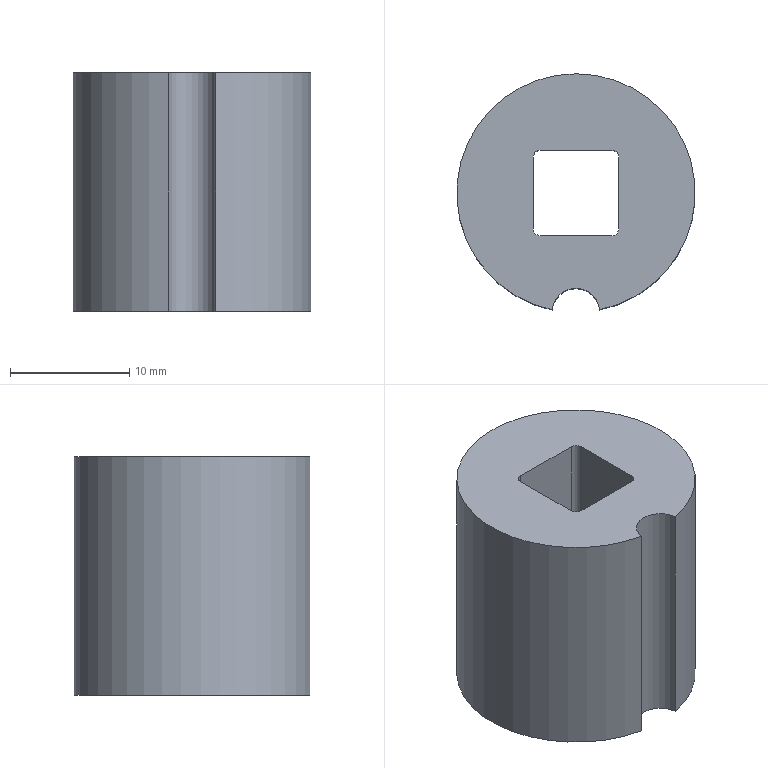Part | NX | features solid 2 | 1 solid | 14 faces | box 20 x 19.802 x 20 mm | volume 4258 mm3 | plane 7 | cylinder 7 | commonest cylinder face diameters 1.17 x4 4 x1 12.6 x1 20 x1
STEP:
#1=CARTESIAN_POINT('',(681.984,-23.915,28.23));
#2=VERTEX_POINT('',#1);
#3=CARTESIAN_POINT('',(678.004,-23.911,28.23));
#4=VERTEX_POINT('',#3);
#5=CARTESIAN_POINT('',(679.993,-24.113,28.23));
#6=DIRECTION('',(0.,0.,1.));
#7=DIRECTION('',(0.001096,1.,0.));
#8=AXIS2_PLACEMENT_3D('',#5,#6,#7);
#9=CIRCLE('',#8,2.);
#10=EDGE_CURVE('',#2,#4,#9,.T.);
#11=ORIENTED_EDGE('',*,*,#10,.F.);
#12=CARTESIAN_POINT('',(680.004,-14.113,28.23));
#13=DIRECTION('',(0.,0.,1.));
#14=DIRECTION('',(0.001096,1.,0.));
#15=AXIS2_PLACEMENT_3D('',#12,#13,#14);
#16=CIRCLE('',#15,10.);
#17=EDGE_CURVE('',#2,#4,#16,.T.);
#18=ORIENTED_EDGE('',*,*,#17,.T.);
#19=EDGE_LOOP('',(#11,#18));
#20=FACE_BOUND('',#19,.T.);
#21=CARTESIAN_POINT('',(677.001,-17.695,28.23));
#22=VERTEX_POINT('',#21);
#23=CARTESIAN_POINT('',(676.416,-17.109,28.23));
#24=VERTEX_POINT('',#23);
#25=CARTESIAN_POINT('',(677.001,-17.11,28.23));
#26=DIRECTION('',(0.,0.,-1.));
#27=DIRECTION('',(-1.,0.,0.));
#28=AXIS2_PLACEMENT_3D('',#25,#26,#27);
#29=CIRCLE('',#28,0.585);
#30=EDGE_CURVE('',#22,#24,#29,.T.);
#31=ORIENTED_EDGE('',*,*,#30,.T.);
#32=CARTESIAN_POINT('',(676.423,-11.109,28.23));
#33=VERTEX_POINT('',#32);
#34=CARTESIAN_POINT('',(676.419,-14.109,28.23));
#35=DIRECTION('',(-0.001096,-1.,0.));
#36=VECTOR('',#35,1000.);
#37=LINE('',#34,#36);
#38=EDGE_CURVE('',#33,#24,#37,.T.);
#39=ORIENTED_EDGE('',*,*,#38,.F.);
#40=CARTESIAN_POINT('',(677.008,-10.525,28.23));
#41=VERTEX_POINT('',#40);
#42=CARTESIAN_POINT('',(677.008,-11.11,28.23));
#43=DIRECTION('',(0.,0.,-1.));
#44=DIRECTION('',(-1.,0.,0.));
#45=AXIS2_PLACEMENT_3D('',#42,#43,#44);
#46=CIRCLE('',#45,0.585);
#47=EDGE_CURVE('',#33,#41,#46,.T.);
#48=ORIENTED_EDGE('',*,*,#47,.T.);
#49=CARTESIAN_POINT('',(683.008,-10.531,28.23));
#50=VERTEX_POINT('',#49);
#51=CARTESIAN_POINT('',(680.008,-10.528,28.23));
#52=DIRECTION('',(-1.,0.001096,0.));
#53=VECTOR('',#52,1000.);
#54=LINE('',#51,#53);
#55=EDGE_CURVE('',#50,#41,#54,.T.);
#56=ORIENTED_EDGE('',*,*,#55,.F.);
#57=CARTESIAN_POINT('',(683.593,-11.117,28.23));
#58=VERTEX_POINT('',#57);
#59=CARTESIAN_POINT('',(683.008,-11.116,28.23));
#60=DIRECTION('',(0.,0.,-1.));
#61=DIRECTION('',(-1.,0.,0.));
#62=AXIS2_PLACEMENT_3D('',#59,#60,#61);
#63=CIRCLE('',#62,0.585);
#64=EDGE_CURVE('',#50,#58,#63,.T.);
#65=ORIENTED_EDGE('',*,*,#64,.T.);
#66=CARTESIAN_POINT('',(683.586,-17.117,28.23));
#67=VERTEX_POINT('',#66);
#68=CARTESIAN_POINT('',(683.589,-14.117,28.23));
#69=DIRECTION('',(0.001096,1.,0.));
#70=VECTOR('',#69,1000.);
#71=LINE('',#68,#70);
#72=EDGE_CURVE('',#67,#58,#71,.T.);
#73=ORIENTED_EDGE('',*,*,#72,.F.);
#74=CARTESIAN_POINT('',(683.001,-17.701,28.23));
#75=VERTEX_POINT('',#74);
#76=CARTESIAN_POINT('',(683.001,-17.116,28.23));
#77=DIRECTION('',(0.,0.,-1.));
#78=DIRECTION('',(-1.,0.,0.));
#79=AXIS2_PLACEMENT_3D('',#76,#77,#78);
#80=CIRCLE('',#79,0.585);
#81=EDGE_CURVE('',#67,#75,#80,.T.);
#82=ORIENTED_EDGE('',*,*,#81,.T.);
#83=CARTESIAN_POINT('',(680.001,-17.698,28.23));
#84=DIRECTION('',(1.,-0.001096,0.));
#85=VECTOR('',#84,1000.);
#86=LINE('',#83,#85);
#87=EDGE_CURVE('',#22,#75,#86,.T.);
#88=ORIENTED_EDGE('',*,*,#87,.F.);
#89=EDGE_LOOP('',(#31,#39,#48,#56,#65,#73,#82,#88));
#90=FACE_BOUND('',#89,.T.);
#91=CARTESIAN_POINT('',(680.004,-14.113,28.23));
#92=DIRECTION('',(0.,0.,1.));
#93=DIRECTION('',(-0.001096,-1.,0.));
#94=AXIS2_PLACEMENT_3D('',#91,#92,#93);
#95=PLANE('',#94);
#96=ADVANCED_FACE('',(#20,#90),#95,.T.);
#97=CARTESIAN_POINT('',(678.004,-23.911,8.23));
#98=VERTEX_POINT('',#97);
#99=CARTESIAN_POINT('',(681.984,-23.915,8.23));
#100=VERTEX_POINT('',#99);
#101=CARTESIAN_POINT('',(679.993,-24.113,8.23));
#102=DIRECTION('',(0.,0.,-1.));
#103=DIRECTION('',(-0.001096,-1.,0.));
#104=AXIS2_PLACEMENT_3D('',#101,#102,#103);
#105=CIRCLE('',#104,2.);
#106=EDGE_CURVE('',#98,#100,#105,.T.);
#107=ORIENTED_EDGE('',*,*,#106,.F.);
#108=CARTESIAN_POINT('',(680.004,-14.113,8.23));
#109=DIRECTION('',(0.,0.,-1.));
#110=DIRECTION('',(-0.001096,-1.,0.));
#111=AXIS2_PLACEMENT_3D('',#108,#109,#110);
#112=CIRCLE('',#111,10.);
#113=EDGE_CURVE('',#98,#100,#112,.T.);
#114=ORIENTED_EDGE('',*,*,#113,.T.);
#115=EDGE_LOOP('',(#107,#114));
#116=FACE_BOUND('',#115,.T.);
#117=CARTESIAN_POINT('',(679.998,-20.413,8.23));
#118=VERTEX_POINT('',#117);
#119=CARTESIAN_POINT('',(680.004,-14.113,8.23));
#120=DIRECTION('',(0.,0.,-1.));
#121=DIRECTION('',(-0.001096,-1.,0.));
#122=AXIS2_PLACEMENT_3D('',#119,#120,#121);
#123=CIRCLE('',#122,6.3);
#124=EDGE_CURVE('',#118,#118,#123,.T.);
#125=ORIENTED_EDGE('',*,*,#124,.F.);
#126=EDGE_LOOP('',(#125));
#127=FACE_BOUND('',#126,.T.);
#128=CARTESIAN_POINT('',(680.004,-14.113,8.23));
#129=DIRECTION('',(0.,0.,-1.));
#130=DIRECTION('',(0.001096,1.,0.));
#131=AXIS2_PLACEMENT_3D('',#128,#129,#130);
#132=PLANE('',#131);
#133=ADVANCED_FACE('',(#116,#127),#132,.T.);
#134=CARTESIAN_POINT('',(678.004,-23.911,18.23));
#135=DIRECTION('',(0.,0.,1.));
#136=VECTOR('',#135,1000.);
#137=LINE('',#134,#136);
#138=EDGE_CURVE('',#98,#4,#137,.T.);
#139=ORIENTED_EDGE('',*,*,#138,.T.);
#140=ORIENTED_EDGE('',*,*,#17,.F.);
#141=CARTESIAN_POINT('',(681.984,-23.915,18.23));
#142=DIRECTION('',(0.,0.,1.));
#143=VECTOR('',#142,1000.);
#144=LINE('',#141,#143);
#145=EDGE_CURVE('',#2,#100,#144,.F.);
#146=ORIENTED_EDGE('',*,*,#145,.T.);
#147=ORIENTED_EDGE('',*,*,#113,.F.);
#148=EDGE_LOOP('',(#139,#140,#146,#147));
#149=FACE_BOUND('',#148,.T.);
#150=CARTESIAN_POINT('',(680.004,-14.113,8.23));
#151=DIRECTION('',(0.,0.,1.));
#152=DIRECTION('',(-0.001096,-1.,0.));
#153=AXIS2_PLACEMENT_3D('',#150,#151,#152);
#154=CYLINDRICAL_SURFACE('',#153,10.);
#155=ADVANCED_FACE('',(#149),#154,.T.);
#156=CARTESIAN_POINT('',(683.001,-17.701,20.23));
#157=VERTEX_POINT('',#156);
#158=CARTESIAN_POINT('',(677.001,-17.695,20.23));
#159=VERTEX_POINT('',#158);
#160=CARTESIAN_POINT('',(680.001,-17.698,20.23));
#161=DIRECTION('',(-1.,0.001096,0.));
#162=VECTOR('',#161,1000.);
#163=LINE('',#160,#162);
#164=EDGE_CURVE('',#157,#159,#163,.T.);
#165=ORIENTED_EDGE('',*,*,#164,.F.);
#166=CARTESIAN_POINT('',(683.586,-17.117,20.23));
#167=VERTEX_POINT('',#166);
#168=CARTESIAN_POINT('',(683.001,-17.116,20.23));
#169=DIRECTION('',(0.,0.,1.));
#170=DIRECTION('',(1.,0.,0.));
#171=AXIS2_PLACEMENT_3D('',#168,#169,#170);
#172=CIRCLE('',#171,0.585);
#173=EDGE_CURVE('',#157,#167,#172,.T.);
#174=ORIENTED_EDGE('',*,*,#173,.T.);
#175=CARTESIAN_POINT('',(683.593,-11.117,20.23));
#176=VERTEX_POINT('',#175);
#177=CARTESIAN_POINT('',(683.589,-14.117,20.23));
#178=DIRECTION('',(-0.001096,-1.,0.));
#179=VECTOR('',#178,1000.);
#180=LINE('',#177,#179);
#181=EDGE_CURVE('',#176,#167,#180,.T.);
#182=ORIENTED_EDGE('',*,*,#181,.F.);
#183=CARTESIAN_POINT('',(683.008,-10.531,20.23));
#184=VERTEX_POINT('',#183);
#185=CARTESIAN_POINT('',(683.008,-11.116,20.23));
#186=DIRECTION('',(0.,0.,1.));
#187=DIRECTION('',(1.,0.,0.));
#188=AXIS2_PLACEMENT_3D('',#185,#186,#187);
#189=CIRCLE('',#188,0.585);
#190=EDGE_CURVE('',#176,#184,#189,.T.);
#191=ORIENTED_EDGE('',*,*,#190,.T.);
#192=CARTESIAN_POINT('',(677.008,-10.525,20.23));
#193=VERTEX_POINT('',#192);
#194=CARTESIAN_POINT('',(680.008,-10.528,20.23));
#195=DIRECTION('',(1.,-0.001096,0.));
#196=VECTOR('',#195,1000.);
#197=LINE('',#194,#196);
#198=EDGE_CURVE('',#193,#184,#197,.T.);
#199=ORIENTED_EDGE('',*,*,#198,.F.);
#200=CARTESIAN_POINT('',(676.423,-11.109,20.23));
#201=VERTEX_POINT('',#200);
#202=CARTESIAN_POINT('',(677.008,-11.11,20.23));
#203=DIRECTION('',(0.,0.,1.));
#204=DIRECTION('',(1.,0.,0.));
#205=AXIS2_PLACEMENT_3D('',#202,#203,#204);
#206=CIRCLE('',#205,0.585);
#207=EDGE_CURVE('',#193,#201,#206,.T.);
#208=ORIENTED_EDGE('',*,*,#207,.T.);
#209=CARTESIAN_POINT('',(676.416,-17.109,20.23));
#210=VERTEX_POINT('',#209);
#211=CARTESIAN_POINT('',(676.419,-14.109,20.23));
#212=DIRECTION('',(0.001096,1.,0.));
#213=VECTOR('',#212,1000.);
#214=LINE('',#211,#213);
#215=EDGE_CURVE('',#210,#201,#214,.T.);
#216=ORIENTED_EDGE('',*,*,#215,.F.);
#217=CARTESIAN_POINT('',(677.001,-17.11,20.23));
#218=DIRECTION('',(0.,0.,1.));
#219=DIRECTION('',(1.,0.,0.));
#220=AXIS2_PLACEMENT_3D('',#217,#218,#219);
#221=CIRCLE('',#220,0.585);
#222=EDGE_CURVE('',#210,#159,#221,.T.);
#223=ORIENTED_EDGE('',*,*,#222,.T.);
#224=EDGE_LOOP('',(#165,#174,#182,#191,#199,#208,#216,#223));
#225=FACE_BOUND('',#224,.T.);
#226=CARTESIAN_POINT('',(680.011,-7.813,20.23));
#227=VERTEX_POINT('',#226);
#228=CARTESIAN_POINT('',(680.004,-14.113,20.23));
#229=DIRECTION('',(0.,0.,1.));
#230=DIRECTION('',(0.001096,1.,0.));
#231=AXIS2_PLACEMENT_3D('',#228,#229,#230);
#232=CIRCLE('',#231,6.3);
#233=EDGE_CURVE('',#227,#227,#232,.T.);
#234=ORIENTED_EDGE('',*,*,#233,.F.);
#235=EDGE_LOOP('',(#234));
#236=FACE_BOUND('',#235,.T.);
#237=CARTESIAN_POINT('',(680.004,-14.113,20.23));
#238=DIRECTION('',(0.,0.,1.));
#239=DIRECTION('',(-0.001096,-1.,0.));
#240=AXIS2_PLACEMENT_3D('',#237,#238,#239);
#241=PLANE('',#240);
#242=ADVANCED_FACE('',(#225,#236),#241,.F.);
#243=ORIENTED_EDGE('',*,*,#233,.T.);
#244=EDGE_LOOP('',(#243));
#245=FACE_BOUND('',#244,.T.);
#246=ORIENTED_EDGE('',*,*,#124,.T.);
#247=EDGE_LOOP('',(#246));
#248=FACE_BOUND('',#247,.T.);
#249=CARTESIAN_POINT('',(680.004,-14.113,8.23));
#250=DIRECTION('',(0.,0.,1.));
#251=DIRECTION('',(-0.001096,-1.,0.));
#252=AXIS2_PLACEMENT_3D('',#249,#250,#251);
#253=CYLINDRICAL_SURFACE('',#252,6.3);
#254=ADVANCED_FACE('',(#245,#248),#253,.F.);
#255=ORIENTED_EDGE('',*,*,#181,.T.);
#256=CARTESIAN_POINT('',(683.586,-17.117,20.23));
#257=DIRECTION('',(0.,0.,1.));
#258=VECTOR('',#257,1000.);
#259=LINE('',#256,#258);
#260=EDGE_CURVE('',#167,#67,#259,.T.);
#261=ORIENTED_EDGE('',*,*,#260,.T.);
#262=ORIENTED_EDGE('',*,*,#72,.T.);
#263=CARTESIAN_POINT('',(683.593,-11.117,20.23));
#264=DIRECTION('',(0.,0.,1.));
#265=VECTOR('',#264,1000.);
#266=LINE('',#263,#265);
#267=EDGE_CURVE('',#58,#176,#266,.F.);
#268=ORIENTED_EDGE('',*,*,#267,.T.);
#269=EDGE_LOOP('',(#255,#261,#262,#268));
#270=FACE_BOUND('',#269,.T.);
#271=CARTESIAN_POINT('',(683.589,-14.117,20.23));
#272=DIRECTION('',(1.,-0.001096,0.));
#273=DIRECTION('',(0.,0.,-1.));
#274=AXIS2_PLACEMENT_3D('',#271,#272,#273);
#275=PLANE('',#274);
#276=ADVANCED_FACE('',(#270),#275,.F.);
#277=ORIENTED_EDGE('',*,*,#55,.T.);
#278=CARTESIAN_POINT('',(677.008,-10.525,20.23));
#279=DIRECTION('',(0.,0.,1.));
#280=VECTOR('',#279,1000.);
#281=LINE('',#278,#280);
#282=EDGE_CURVE('',#41,#193,#281,.F.);
#283=ORIENTED_EDGE('',*,*,#282,.T.);
#284=ORIENTED_EDGE('',*,*,#198,.T.);
#285=CARTESIAN_POINT('',(683.008,-10.531,20.23));
#286=DIRECTION('',(0.,0.,1.));
#287=VECTOR('',#286,1000.);
#288=LINE('',#285,#287);
#289=EDGE_CURVE('',#184,#50,#288,.T.);
#290=ORIENTED_EDGE('',*,*,#289,.T.);
#291=EDGE_LOOP('',(#277,#283,#284,#290));
#292=FACE_BOUND('',#291,.T.);
#293=CARTESIAN_POINT('',(680.008,-10.528,20.23));
#294=DIRECTION('',(0.001096,1.,0.));
#295=DIRECTION('',(0.,0.,1.));
#296=AXIS2_PLACEMENT_3D('',#293,#294,#295);
#297=PLANE('',#296);
#298=ADVANCED_FACE('',(#292),#297,.F.);
#299=ORIENTED_EDGE('',*,*,#38,.T.);
#300=CARTESIAN_POINT('',(676.416,-17.109,20.23));
#301=DIRECTION('',(0.,0.,1.));
#302=VECTOR('',#301,1000.);
#303=LINE('',#300,#302);
#304=EDGE_CURVE('',#24,#210,#303,.F.);
#305=ORIENTED_EDGE('',*,*,#304,.T.);
#306=ORIENTED_EDGE('',*,*,#215,.T.);
#307=CARTESIAN_POINT('',(676.423,-11.109,20.23));
#308=DIRECTION('',(0.,0.,1.));
#309=VECTOR('',#308,1000.);
#310=LINE('',#307,#309);
#311=EDGE_CURVE('',#201,#33,#310,.T.);
#312=ORIENTED_EDGE('',*,*,#311,.T.);
#313=EDGE_LOOP('',(#299,#305,#306,#312));
#314=FACE_BOUND('',#313,.T.);
#315=CARTESIAN_POINT('',(676.419,-14.109,20.23));
#316=DIRECTION('',(-1.,0.001096,0.));
#317=DIRECTION('',(0.,0.,1.));
#318=AXIS2_PLACEMENT_3D('',#315,#316,#317);
#319=PLANE('',#318);
#320=ADVANCED_FACE('',(#314),#319,.F.);
#321=ORIENTED_EDGE('',*,*,#87,.T.);
#322=CARTESIAN_POINT('',(683.001,-17.701,20.23));
#323=DIRECTION('',(0.,0.,1.));
#324=VECTOR('',#323,1000.);
#325=LINE('',#322,#324);
#326=EDGE_CURVE('',#75,#157,#325,.F.);
#327=ORIENTED_EDGE('',*,*,#326,.T.);
#328=ORIENTED_EDGE('',*,*,#164,.T.);
#329=CARTESIAN_POINT('',(677.001,-17.695,20.23));
#330=DIRECTION('',(0.,0.,1.));
#331=VECTOR('',#330,1000.);
#332=LINE('',#329,#331);
#333=EDGE_CURVE('',#159,#22,#332,.T.);
#334=ORIENTED_EDGE('',*,*,#333,.T.);
#335=EDGE_LOOP('',(#321,#327,#328,#334));
#336=FACE_BOUND('',#335,.T.);
#337=CARTESIAN_POINT('',(680.001,-17.698,20.23));
#338=DIRECTION('',(-0.001096,-1.,0.));
#339=DIRECTION('',(0.,0.,-1.));
#340=AXIS2_PLACEMENT_3D('',#337,#338,#339);
#341=PLANE('',#340);
#342=ADVANCED_FACE('',(#336),#341,.F.);
#343=ORIENTED_EDGE('',*,*,#173,.F.);
#344=ORIENTED_EDGE('',*,*,#326,.F.);
#345=ORIENTED_EDGE('',*,*,#81,.F.);
#346=ORIENTED_EDGE('',*,*,#260,.F.);
#347=EDGE_LOOP('',(#343,#344,#345,#346));
#348=FACE_BOUND('',#347,.T.);
#349=CARTESIAN_POINT('',(683.001,-17.116,20.23));
#350=DIRECTION('',(0.,0.,1.));
#351=DIRECTION('',(-1.,0.,0.));
#352=AXIS2_PLACEMENT_3D('',#349,#350,#351);
#353=CYLINDRICAL_SURFACE('',#352,0.585);
#354=ADVANCED_FACE('',(#348),#353,.F.);
#355=ORIENTED_EDGE('',*,*,#222,.F.);
#356=ORIENTED_EDGE('',*,*,#304,.F.);
#357=ORIENTED_EDGE('',*,*,#30,.F.);
#358=ORIENTED_EDGE('',*,*,#333,.F.);
#359=EDGE_LOOP('',(#355,#356,#357,#358));
#360=FACE_BOUND('',#359,.T.);
#361=CARTESIAN_POINT('',(677.001,-17.11,20.23));
#362=DIRECTION('',(0.,0.,1.));
#363=DIRECTION('',(-1.,0.,0.));
#364=AXIS2_PLACEMENT_3D('',#361,#362,#363);
#365=CYLINDRICAL_SURFACE('',#364,0.585);
#366=ADVANCED_FACE('',(#360),#365,.F.);
#367=ORIENTED_EDGE('',*,*,#207,.F.);
#368=ORIENTED_EDGE('',*,*,#282,.F.);
#369=ORIENTED_EDGE('',*,*,#47,.F.);
#370=ORIENTED_EDGE('',*,*,#311,.F.);
#371=EDGE_LOOP('',(#367,#368,#369,#370));
#372=FACE_BOUND('',#371,.T.);
#373=CARTESIAN_POINT('',(677.008,-11.11,20.23));
#374=DIRECTION('',(0.,0.,1.));
#375=DIRECTION('',(-1.,0.,0.));
#376=AXIS2_PLACEMENT_3D('',#373,#374,#375);
#377=CYLINDRICAL_SURFACE('',#376,0.585);
#378=ADVANCED_FACE('',(#372),#377,.F.);
#379=ORIENTED_EDGE('',*,*,#190,.F.);
#380=ORIENTED_EDGE('',*,*,#267,.F.);
#381=ORIENTED_EDGE('',*,*,#64,.F.);
#382=ORIENTED_EDGE('',*,*,#289,.F.);
#383=EDGE_LOOP('',(#379,#380,#381,#382));
#384=FACE_BOUND('',#383,.T.);
#385=CARTESIAN_POINT('',(683.008,-11.116,20.23));
#386=DIRECTION('',(0.,0.,1.));
#387=DIRECTION('',(-1.,0.,0.));
#388=AXIS2_PLACEMENT_3D('',#385,#386,#387);
#389=CYLINDRICAL_SURFACE('',#388,0.585);
#390=ADVANCED_FACE('',(#384),#389,.F.);
#391=ORIENTED_EDGE('',*,*,#138,.F.);
#392=ORIENTED_EDGE('',*,*,#106,.T.);
#393=ORIENTED_EDGE('',*,*,#145,.F.);
#394=ORIENTED_EDGE('',*,*,#10,.T.);
#395=EDGE_LOOP('',(#391,#392,#393,#394));
#396=FACE_BOUND('',#395,.T.);
#397=CARTESIAN_POINT('',(679.993,-24.113,8.23));
#398=DIRECTION('',(0.,0.,1.));
#399=DIRECTION('',(-0.001096,-1.,0.));
#400=AXIS2_PLACEMENT_3D('',#397,#398,#399);
#401=CYLINDRICAL_SURFACE('',#400,2.);
#402=ADVANCED_FACE('',(#396),#401,.F.);
#403=CLOSED_SHELL('',(#96,#133,#155,#242,#254,#276,#298,#320,#342,#354,#366,#378,#390,#402));
#404=MANIFOLD_SOLID_BREP('',#403);
#405=(LENGTH_UNIT()NAMED_UNIT(*)SI_UNIT(.MILLI.,.METRE.));
#406=UNCERTAINTY_MEASURE_WITH_UNIT(LENGTH_MEASURE(0.00001),#405,'','');
#407=(NAMED_UNIT(*)PLANE_ANGLE_UNIT()SI_UNIT($,.RADIAN.));
#408=(NAMED_UNIT(*)SI_UNIT($,.STERADIAN.)SOLID_ANGLE_UNIT());
#409=(GEOMETRIC_REPRESENTATION_CONTEXT(3)GLOBAL_UNCERTAINTY_ASSIGNED_CONTEXT((#406))GLOBAL_UNIT_ASSIGNED_CONTEXT((#405,#407,#408))REPRESENTATION_CONTEXT('',''));
#410=ADVANCED_BREP_SHAPE_REPRESENTATION('',(#404),#409);